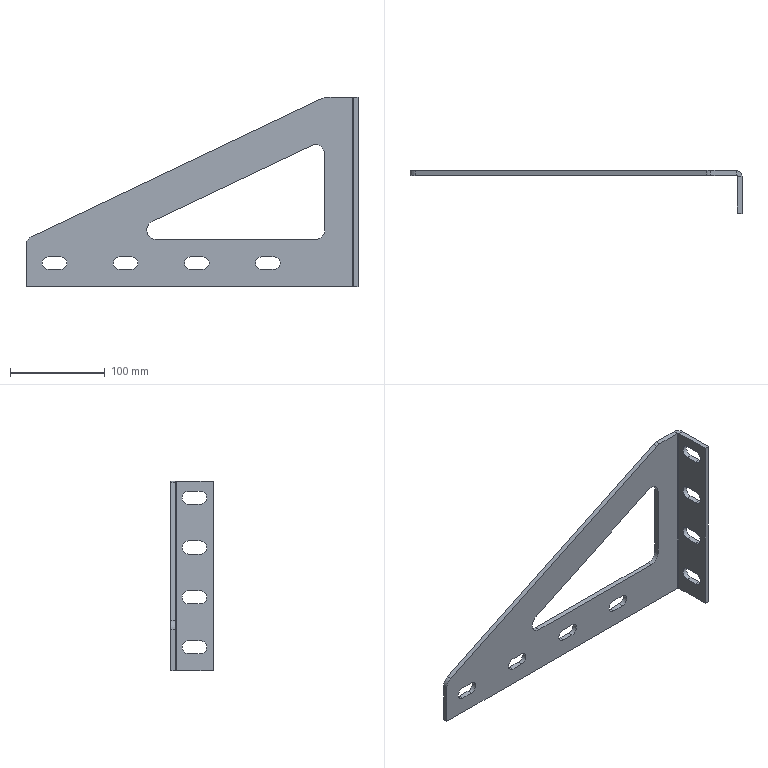Part | SolidWorks | features ICE 8, Fillet 3, FlatPattern 1, SMBaseFlange 1, SheetMetal 1 | 1 solid | 59 faces | box 350 x 45 x 200 mm | volume 201146 mm3 | plane 32 | cylinder 27 | commonest cylinder face diameters 14 x12 13 x8 20 x5 2 x1 12 x1